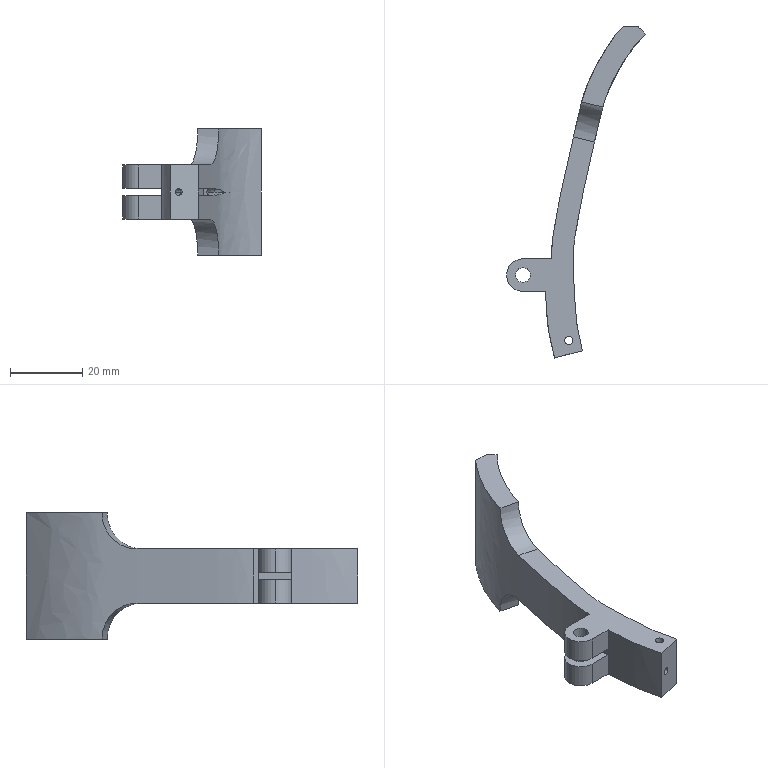Part | SolidWorks | features ICE 6, Fillet 2, Chamfer 1, Extrusion 1, SweepCut 1 | 1 solid | 41 faces | box 38.444 x 92.062 x 35 mm | volume 13126 mm3 | plane 17 | spline 12 | cylinder 12 | commonest cylinder face diameters 4.1 x4 9 x4 2.3 x2 20 x2